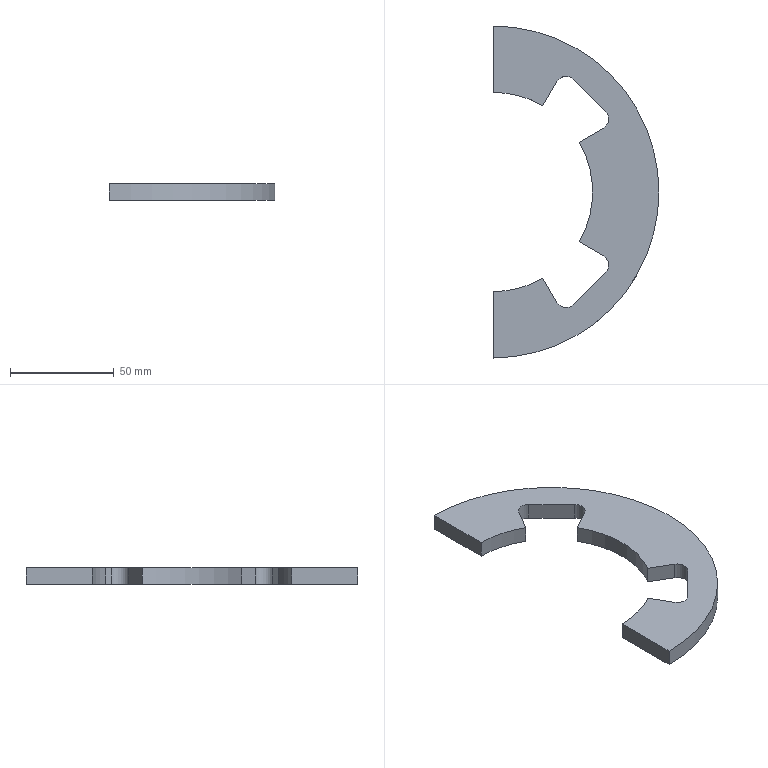Part | SolidWorks | features FlatPattern 1, SMBaseFlange 1, SheetMetal 1 | 1 solid | 18 faces | box 80 x 160 x 8 mm | volume 42936 mm3 | plane 10 | cylinder 8 | commonest cylinder face diameters 10 x4 96 x3 160 x1
STEP:
#1=CARTESIAN_POINT('',(125.,-80.,0.));
#2=VERTEX_POINT('',#1);
#3=CARTESIAN_POINT('',(125.,80.,0.));
#4=VERTEX_POINT('',#3);
#5=CARTESIAN_POINT('',(125.,0.,0.));
#6=DIRECTION('',(0.,0.,1.));
#7=DIRECTION('',(1.,0.,0.));
#8=AXIS2_PLACEMENT_3D('',#5,#6,#7);
#9=CIRCLE('',#8,80.);
#10=EDGE_CURVE('',#2,#4,#9,.T.);
#11=ORIENTED_EDGE('',*,*,#10,.T.);
#12=CARTESIAN_POINT('',(125.,80.,8.));
#13=VERTEX_POINT('',#12);
#14=CARTESIAN_POINT('',(125.,80.,8.));
#15=DIRECTION('',(0.,0.,-1.));
#16=VECTOR('',#15,1000.);
#17=LINE('',#14,#16);
#18=EDGE_CURVE('',#13,#4,#17,.T.);
#19=ORIENTED_EDGE('',*,*,#18,.F.);
#20=CARTESIAN_POINT('',(125.,-80.,8.));
#21=VERTEX_POINT('',#20);
#22=CARTESIAN_POINT('',(125.,0.,8.));
#23=DIRECTION('',(0.,0.,1.));
#24=DIRECTION('',(1.,0.,0.));
#25=AXIS2_PLACEMENT_3D('',#22,#23,#24);
#26=CIRCLE('',#25,80.);
#27=EDGE_CURVE('',#21,#13,#26,.T.);
#28=ORIENTED_EDGE('',*,*,#27,.F.);
#29=CARTESIAN_POINT('',(125.,-80.,8.));
#30=DIRECTION('',(0.,0.,-1.));
#31=VECTOR('',#30,1000.);
#32=LINE('',#29,#31);
#33=EDGE_CURVE('',#21,#2,#32,.T.);
#34=ORIENTED_EDGE('',*,*,#33,.T.);
#35=EDGE_LOOP('',(#11,#19,#28,#34));
#36=FACE_OUTER_BOUND('',#35,.T.);
#37=CARTESIAN_POINT('',(125.,0.,8.));
#38=DIRECTION('',(0.,0.,-1.));
#39=DIRECTION('',(-1.,0.,0.));
#40=AXIS2_PLACEMENT_3D('',#37,#38,#39);
#41=CYLINDRICAL_SURFACE('',#40,80.);
#42=ADVANCED_FACE('',(#36),#41,.T.);
#43=CARTESIAN_POINT('',(125.,48.,0.));
#44=VERTEX_POINT('',#43);
#45=CARTESIAN_POINT('',(125.,80.,0.));
#46=DIRECTION('',(0.,-1.,0.));
#47=VECTOR('',#46,1000.);
#48=LINE('',#45,#47);
#49=EDGE_CURVE('',#4,#44,#48,.T.);
#50=ORIENTED_EDGE('',*,*,#49,.T.);
#51=CARTESIAN_POINT('',(125.,48.,8.));
#52=VERTEX_POINT('',#51);
#53=CARTESIAN_POINT('',(125.,48.,8.));
#54=DIRECTION('',(0.,0.,-1.));
#55=VECTOR('',#54,1000.);
#56=LINE('',#53,#55);
#57=EDGE_CURVE('',#52,#44,#56,.T.);
#58=ORIENTED_EDGE('',*,*,#57,.F.);
#59=CARTESIAN_POINT('',(125.,80.,8.));
#60=DIRECTION('',(0.,-1.,0.));
#61=VECTOR('',#60,1000.);
#62=LINE('',#59,#61);
#63=EDGE_CURVE('',#13,#52,#62,.T.);
#64=ORIENTED_EDGE('',*,*,#63,.F.);
#65=ORIENTED_EDGE('',*,*,#18,.T.);
#66=EDGE_LOOP('',(#50,#58,#64,#65));
#67=FACE_OUTER_BOUND('',#66,.T.);
#68=CARTESIAN_POINT('',(125.,80.,8.));
#69=DIRECTION('',(1.,0.,0.));
#70=DIRECTION('',(0.,0.,-1.));
#71=AXIS2_PLACEMENT_3D('',#68,#69,#70);
#72=PLANE('',#71);
#73=ADVANCED_FACE('',(#67),#72,.F.);
#74=CARTESIAN_POINT('',(149.,41.569,0.));
#75=VERTEX_POINT('',#74);
#76=CARTESIAN_POINT('',(125.,0.,0.));
#77=DIRECTION('',(0.,0.,-1.));
#78=DIRECTION('',(1.,0.,0.));
#79=AXIS2_PLACEMENT_3D('',#76,#77,#78);
#80=CIRCLE('',#79,48.);
#81=EDGE_CURVE('',#44,#75,#80,.T.);
#82=ORIENTED_EDGE('',*,*,#81,.T.);
#83=CARTESIAN_POINT('',(149.,41.569,8.));
#84=VERTEX_POINT('',#83);
#85=CARTESIAN_POINT('',(149.,41.569,8.));
#86=DIRECTION('',(0.,0.,-1.));
#87=VECTOR('',#86,1000.);
#88=LINE('',#85,#87);
#89=EDGE_CURVE('',#84,#75,#88,.T.);
#90=ORIENTED_EDGE('',*,*,#89,.F.);
#91=CARTESIAN_POINT('',(125.,0.,8.));
#92=DIRECTION('',(0.,0.,-1.));
#93=DIRECTION('',(1.,0.,0.));
#94=AXIS2_PLACEMENT_3D('',#91,#92,#93);
#95=CIRCLE('',#94,48.);
#96=EDGE_CURVE('',#52,#84,#95,.T.);
#97=ORIENTED_EDGE('',*,*,#96,.F.);
#98=ORIENTED_EDGE('',*,*,#57,.T.);
#99=EDGE_LOOP('',(#82,#90,#97,#98));
#100=FACE_OUTER_BOUND('',#99,.T.);
#101=CARTESIAN_POINT('',(125.,0.,8.));
#102=DIRECTION('',(0.,0.,-1.));
#103=DIRECTION('',(-1.,0.,0.));
#104=AXIS2_PLACEMENT_3D('',#101,#102,#103);
#105=CYLINDRICAL_SURFACE('',#104,48.);
#106=ADVANCED_FACE('',(#100),#105,.F.);
#107=CARTESIAN_POINT('',(155.742,53.247,0.));
#108=VERTEX_POINT('',#107);
#109=CARTESIAN_POINT('',(155.742,53.247,0.));
#110=DIRECTION('',(0.5,0.866,0.));
#111=VECTOR('',#110,1000.);
#112=LINE('',#109,#111);
#113=EDGE_CURVE('',#75,#108,#112,.T.);
#114=ORIENTED_EDGE('',*,*,#113,.T.);
#115=CARTESIAN_POINT('',(155.742,53.247,8.));
#116=VERTEX_POINT('',#115);
#117=CARTESIAN_POINT('',(155.742,53.247,8.));
#118=DIRECTION('',(0.,0.,-1.));
#119=VECTOR('',#118,1000.);
#120=LINE('',#117,#119);
#121=EDGE_CURVE('',#116,#108,#120,.T.);
#122=ORIENTED_EDGE('',*,*,#121,.F.);
#123=CARTESIAN_POINT('',(155.742,53.247,8.));
#124=DIRECTION('',(0.5,0.866,0.));
#125=VECTOR('',#124,1000.);
#126=LINE('',#123,#125);
#127=EDGE_CURVE('',#84,#116,#126,.T.);
#128=ORIENTED_EDGE('',*,*,#127,.F.);
#129=ORIENTED_EDGE('',*,*,#89,.T.);
#130=EDGE_LOOP('',(#114,#122,#128,#129));
#131=FACE_OUTER_BOUND('',#130,.T.);
#132=CARTESIAN_POINT('',(155.742,53.247,8.));
#133=DIRECTION('',(-0.866,0.5,0.));
#134=DIRECTION('',(-0.5,-0.866,0.));
#135=AXIS2_PLACEMENT_3D('',#132,#133,#134);
#136=PLANE('',#135);
#137=ADVANCED_FACE('',(#131),#136,.F.);
#138=CARTESIAN_POINT('',(163.608,54.282,0.));
#139=VERTEX_POINT('',#138);
#140=CARTESIAN_POINT('',(160.072,50.747,0.));
#141=DIRECTION('',(0.,0.,-1.));
#142=DIRECTION('',(1.,0.,0.));
#143=AXIS2_PLACEMENT_3D('',#140,#141,#142);
#144=CIRCLE('',#143,5.);
#145=EDGE_CURVE('',#108,#139,#144,.T.);
#146=ORIENTED_EDGE('',*,*,#145,.T.);
#147=CARTESIAN_POINT('',(163.608,54.282,8.));
#148=VERTEX_POINT('',#147);
#149=CARTESIAN_POINT('',(163.608,54.282,8.));
#150=DIRECTION('',(0.,0.,-1.));
#151=VECTOR('',#150,1000.);
#152=LINE('',#149,#151);
#153=EDGE_CURVE('',#148,#139,#152,.T.);
#154=ORIENTED_EDGE('',*,*,#153,.F.);
#155=CARTESIAN_POINT('',(160.072,50.747,8.));
#156=DIRECTION('',(0.,0.,-1.));
#157=DIRECTION('',(1.,0.,0.));
#158=AXIS2_PLACEMENT_3D('',#155,#156,#157);
#159=CIRCLE('',#158,5.);
#160=EDGE_CURVE('',#116,#148,#159,.T.);
#161=ORIENTED_EDGE('',*,*,#160,.F.);
#162=ORIENTED_EDGE('',*,*,#121,.T.);
#163=EDGE_LOOP('',(#146,#154,#161,#162));
#164=FACE_OUTER_BOUND('',#163,.T.);
#165=CARTESIAN_POINT('',(160.072,50.747,8.));
#166=DIRECTION('',(0.,0.,-1.));
#167=DIRECTION('',(-1.,0.,0.));
#168=AXIS2_PLACEMENT_3D('',#165,#166,#167);
#169=CYLINDRICAL_SURFACE('',#168,5.);
#170=ADVANCED_FACE('',(#164),#169,.F.);
#171=CARTESIAN_POINT('',(179.282,38.608,0.));
#172=VERTEX_POINT('',#171);
#173=CARTESIAN_POINT('',(163.608,54.282,0.));
#174=DIRECTION('',(0.7071,-0.7071,0.));
#175=VECTOR('',#174,1000.);
#176=LINE('',#173,#175);
#177=EDGE_CURVE('',#139,#172,#176,.T.);
#178=ORIENTED_EDGE('',*,*,#177,.T.);
#179=CARTESIAN_POINT('',(179.282,38.608,8.));
#180=VERTEX_POINT('',#179);
#181=CARTESIAN_POINT('',(179.282,38.608,8.));
#182=DIRECTION('',(0.,0.,-1.));
#183=VECTOR('',#182,1000.);
#184=LINE('',#181,#183);
#185=EDGE_CURVE('',#180,#172,#184,.T.);
#186=ORIENTED_EDGE('',*,*,#185,.F.);
#187=CARTESIAN_POINT('',(163.608,54.282,8.));
#188=DIRECTION('',(0.7071,-0.7071,0.));
#189=VECTOR('',#188,1000.);
#190=LINE('',#187,#189);
#191=EDGE_CURVE('',#148,#180,#190,.T.);
#192=ORIENTED_EDGE('',*,*,#191,.F.);
#193=ORIENTED_EDGE('',*,*,#153,.T.);
#194=EDGE_LOOP('',(#178,#186,#192,#193));
#195=FACE_OUTER_BOUND('',#194,.T.);
#196=CARTESIAN_POINT('',(163.608,54.282,8.));
#197=DIRECTION('',(0.7071,0.7071,0.));
#198=DIRECTION('',(-0.7071,0.7071,0.));
#199=AXIS2_PLACEMENT_3D('',#196,#197,#198);
#200=PLANE('',#199);
#201=ADVANCED_FACE('',(#195),#200,.F.);
#202=CARTESIAN_POINT('',(178.247,30.742,0.));
#203=VERTEX_POINT('',#202);
#204=CARTESIAN_POINT('',(175.747,35.072,0.));
#205=DIRECTION('',(0.,0.,-1.));
#206=DIRECTION('',(1.,0.,0.));
#207=AXIS2_PLACEMENT_3D('',#204,#205,#206);
#208=CIRCLE('',#207,5.);
#209=EDGE_CURVE('',#172,#203,#208,.T.);
#210=ORIENTED_EDGE('',*,*,#209,.T.);
#211=CARTESIAN_POINT('',(178.247,30.742,8.));
#212=VERTEX_POINT('',#211);
#213=CARTESIAN_POINT('',(178.247,30.742,8.));
#214=DIRECTION('',(0.,0.,-1.));
#215=VECTOR('',#214,1000.);
#216=LINE('',#213,#215);
#217=EDGE_CURVE('',#212,#203,#216,.T.);
#218=ORIENTED_EDGE('',*,*,#217,.F.);
#219=CARTESIAN_POINT('',(175.747,35.072,8.));
#220=DIRECTION('',(0.,0.,-1.));
#221=DIRECTION('',(1.,0.,0.));
#222=AXIS2_PLACEMENT_3D('',#219,#220,#221);
#223=CIRCLE('',#222,5.);
#224=EDGE_CURVE('',#180,#212,#223,.T.);
#225=ORIENTED_EDGE('',*,*,#224,.F.);
#226=ORIENTED_EDGE('',*,*,#185,.T.);
#227=EDGE_LOOP('',(#210,#218,#225,#226));
#228=FACE_OUTER_BOUND('',#227,.T.);
#229=CARTESIAN_POINT('',(175.747,35.072,8.));
#230=DIRECTION('',(0.,0.,-1.));
#231=DIRECTION('',(-1.,0.,0.));
#232=AXIS2_PLACEMENT_3D('',#229,#230,#231);
#233=CYLINDRICAL_SURFACE('',#232,5.);
#234=ADVANCED_FACE('',(#228),#233,.F.);
#235=CARTESIAN_POINT('',(166.569,24.,0.));
#236=VERTEX_POINT('',#235);
#237=CARTESIAN_POINT('',(166.569,24.,0.));
#238=DIRECTION('',(-0.866,-0.5,0.));
#239=VECTOR('',#238,1000.);
#240=LINE('',#237,#239);
#241=EDGE_CURVE('',#203,#236,#240,.T.);
#242=ORIENTED_EDGE('',*,*,#241,.T.);
#243=CARTESIAN_POINT('',(166.569,24.,8.));
#244=VERTEX_POINT('',#243);
#245=CARTESIAN_POINT('',(166.569,24.,8.));
#246=DIRECTION('',(0.,0.,-1.));
#247=VECTOR('',#246,1000.);
#248=LINE('',#245,#247);
#249=EDGE_CURVE('',#244,#236,#248,.T.);
#250=ORIENTED_EDGE('',*,*,#249,.F.);
#251=CARTESIAN_POINT('',(166.569,24.,8.));
#252=DIRECTION('',(-0.866,-0.5,0.));
#253=VECTOR('',#252,1000.);
#254=LINE('',#251,#253);
#255=EDGE_CURVE('',#212,#244,#254,.T.);
#256=ORIENTED_EDGE('',*,*,#255,.F.);
#257=ORIENTED_EDGE('',*,*,#217,.T.);
#258=EDGE_LOOP('',(#242,#250,#256,#257));
#259=FACE_OUTER_BOUND('',#258,.T.);
#260=CARTESIAN_POINT('',(166.569,24.,8.));
#261=DIRECTION('',(0.5,-0.866,0.));
#262=DIRECTION('',(0.866,0.5,0.));
#263=AXIS2_PLACEMENT_3D('',#260,#261,#262);
#264=PLANE('',#263);
#265=ADVANCED_FACE('',(#259),#264,.F.);
#266=CARTESIAN_POINT('',(166.569,-24.,0.));
#267=VERTEX_POINT('',#266);
#268=CARTESIAN_POINT('',(125.,0.,0.));
#269=DIRECTION('',(0.,0.,-1.));
#270=DIRECTION('',(1.,0.,0.));
#271=AXIS2_PLACEMENT_3D('',#268,#269,#270);
#272=CIRCLE('',#271,48.);
#273=EDGE_CURVE('',#236,#267,#272,.T.);
#274=ORIENTED_EDGE('',*,*,#273,.T.);
#275=CARTESIAN_POINT('',(166.569,-24.,8.));
#276=VERTEX_POINT('',#275);
#277=CARTESIAN_POINT('',(166.569,-24.,8.));
#278=DIRECTION('',(0.,0.,-1.));
#279=VECTOR('',#278,1000.);
#280=LINE('',#277,#279);
#281=EDGE_CURVE('',#276,#267,#280,.T.);
#282=ORIENTED_EDGE('',*,*,#281,.F.);
#283=CARTESIAN_POINT('',(125.,0.,8.));
#284=DIRECTION('',(0.,0.,-1.));
#285=DIRECTION('',(1.,0.,0.));
#286=AXIS2_PLACEMENT_3D('',#283,#284,#285);
#287=CIRCLE('',#286,48.);
#288=EDGE_CURVE('',#244,#276,#287,.T.);
#289=ORIENTED_EDGE('',*,*,#288,.F.);
#290=ORIENTED_EDGE('',*,*,#249,.T.);
#291=EDGE_LOOP('',(#274,#282,#289,#290));
#292=FACE_OUTER_BOUND('',#291,.T.);
#293=CARTESIAN_POINT('',(125.,0.,8.));
#294=DIRECTION('',(0.,0.,-1.));
#295=DIRECTION('',(-1.,0.,0.));
#296=AXIS2_PLACEMENT_3D('',#293,#294,#295);
#297=CYLINDRICAL_SURFACE('',#296,48.);
#298=ADVANCED_FACE('',(#292),#297,.F.);
#299=CARTESIAN_POINT('',(178.247,-30.742,0.));
#300=VERTEX_POINT('',#299);
#301=CARTESIAN_POINT('',(166.569,-24.,0.));
#302=DIRECTION('',(0.866,-0.5,0.));
#303=VECTOR('',#302,1000.);
#304=LINE('',#301,#303);
#305=EDGE_CURVE('',#267,#300,#304,.T.);
#306=ORIENTED_EDGE('',*,*,#305,.T.);
#307=CARTESIAN_POINT('',(178.247,-30.742,8.));
#308=VERTEX_POINT('',#307);
#309=CARTESIAN_POINT('',(178.247,-30.742,8.));
#310=DIRECTION('',(0.,0.,-1.));
#311=VECTOR('',#310,1000.);
#312=LINE('',#309,#311);
#313=EDGE_CURVE('',#308,#300,#312,.T.);
#314=ORIENTED_EDGE('',*,*,#313,.F.);
#315=CARTESIAN_POINT('',(166.569,-24.,8.));
#316=DIRECTION('',(0.866,-0.5,0.));
#317=VECTOR('',#316,1000.);
#318=LINE('',#315,#317);
#319=EDGE_CURVE('',#276,#308,#318,.T.);
#320=ORIENTED_EDGE('',*,*,#319,.F.);
#321=ORIENTED_EDGE('',*,*,#281,.T.);
#322=EDGE_LOOP('',(#306,#314,#320,#321));
#323=FACE_OUTER_BOUND('',#322,.T.);
#324=CARTESIAN_POINT('',(166.569,-24.,8.));
#325=DIRECTION('',(0.5,0.866,0.));
#326=DIRECTION('',(-0.866,0.5,0.));
#327=AXIS2_PLACEMENT_3D('',#324,#325,#326);
#328=PLANE('',#327);
#329=ADVANCED_FACE('',(#323),#328,.F.);
#330=CARTESIAN_POINT('',(179.282,-38.608,0.));
#331=VERTEX_POINT('',#330);
#332=CARTESIAN_POINT('',(175.747,-35.072,0.));
#333=DIRECTION('',(0.,0.,-1.));
#334=DIRECTION('',(-1.,0.,0.));
#335=AXIS2_PLACEMENT_3D('',#332,#333,#334);
#336=CIRCLE('',#335,5.);
#337=EDGE_CURVE('',#300,#331,#336,.T.);
#338=ORIENTED_EDGE('',*,*,#337,.T.);
#339=CARTESIAN_POINT('',(179.282,-38.608,8.));
#340=VERTEX_POINT('',#339);
#341=CARTESIAN_POINT('',(179.282,-38.608,8.));
#342=DIRECTION('',(0.,0.,-1.));
#343=VECTOR('',#342,1000.);
#344=LINE('',#341,#343);
#345=EDGE_CURVE('',#340,#331,#344,.T.);
#346=ORIENTED_EDGE('',*,*,#345,.F.);
#347=CARTESIAN_POINT('',(175.747,-35.072,8.));
#348=DIRECTION('',(0.,0.,-1.));
#349=DIRECTION('',(-1.,0.,0.));
#350=AXIS2_PLACEMENT_3D('',#347,#348,#349);
#351=CIRCLE('',#350,5.);
#352=EDGE_CURVE('',#308,#340,#351,.T.);
#353=ORIENTED_EDGE('',*,*,#352,.F.);
#354=ORIENTED_EDGE('',*,*,#313,.T.);
#355=EDGE_LOOP('',(#338,#346,#353,#354));
#356=FACE_OUTER_BOUND('',#355,.T.);
#357=CARTESIAN_POINT('',(175.747,-35.072,8.));
#358=DIRECTION('',(0.,0.,-1.));
#359=DIRECTION('',(-1.,0.,0.));
#360=AXIS2_PLACEMENT_3D('',#357,#358,#359);
#361=CYLINDRICAL_SURFACE('',#360,5.);
#362=ADVANCED_FACE('',(#356),#361,.F.);
#363=CARTESIAN_POINT('',(163.608,-54.282,0.));
#364=VERTEX_POINT('',#363);
#365=CARTESIAN_POINT('',(163.608,-54.282,0.));
#366=DIRECTION('',(-0.7071,-0.7071,0.));
#367=VECTOR('',#366,1000.);
#368=LINE('',#365,#367);
#369=EDGE_CURVE('',#331,#364,#368,.T.);
#370=ORIENTED_EDGE('',*,*,#369,.T.);
#371=CARTESIAN_POINT('',(163.608,-54.282,8.));
#372=VERTEX_POINT('',#371);
#373=CARTESIAN_POINT('',(163.608,-54.282,8.));
#374=DIRECTION('',(0.,0.,-1.));
#375=VECTOR('',#374,1000.);
#376=LINE('',#373,#375);
#377=EDGE_CURVE('',#372,#364,#376,.T.);
#378=ORIENTED_EDGE('',*,*,#377,.F.);
#379=CARTESIAN_POINT('',(163.608,-54.282,8.));
#380=DIRECTION('',(-0.7071,-0.7071,0.));
#381=VECTOR('',#380,1000.);
#382=LINE('',#379,#381);
#383=EDGE_CURVE('',#340,#372,#382,.T.);
#384=ORIENTED_EDGE('',*,*,#383,.F.);
#385=ORIENTED_EDGE('',*,*,#345,.T.);
#386=EDGE_LOOP('',(#370,#378,#384,#385));
#387=FACE_OUTER_BOUND('',#386,.T.);
#388=CARTESIAN_POINT('',(163.608,-54.282,8.));
#389=DIRECTION('',(0.7071,-0.7071,0.));
#390=DIRECTION('',(0.7071,0.7071,0.));
#391=AXIS2_PLACEMENT_3D('',#388,#389,#390);
#392=PLANE('',#391);
#393=ADVANCED_FACE('',(#387),#392,.F.);
#394=CARTESIAN_POINT('',(155.742,-53.247,0.));
#395=VERTEX_POINT('',#394);
#396=CARTESIAN_POINT('',(160.072,-50.747,0.));
#397=DIRECTION('',(0.,0.,-1.));
#398=DIRECTION('',(-1.,0.,0.));
#399=AXIS2_PLACEMENT_3D('',#396,#397,#398);
#400=CIRCLE('',#399,5.);
#401=EDGE_CURVE('',#364,#395,#400,.T.);
#402=ORIENTED_EDGE('',*,*,#401,.T.);
#403=CARTESIAN_POINT('',(155.742,-53.247,8.));
#404=VERTEX_POINT('',#403);
#405=CARTESIAN_POINT('',(155.742,-53.247,8.));
#406=DIRECTION('',(0.,0.,-1.));
#407=VECTOR('',#406,1000.);
#408=LINE('',#405,#407);
#409=EDGE_CURVE('',#404,#395,#408,.T.);
#410=ORIENTED_EDGE('',*,*,#409,.F.);
#411=CARTESIAN_POINT('',(160.072,-50.747,8.));
#412=DIRECTION('',(0.,0.,-1.));
#413=DIRECTION('',(-1.,0.,0.));
#414=AXIS2_PLACEMENT_3D('',#411,#412,#413);
#415=CIRCLE('',#414,5.);
#416=EDGE_CURVE('',#372,#404,#415,.T.);
#417=ORIENTED_EDGE('',*,*,#416,.F.);
#418=ORIENTED_EDGE('',*,*,#377,.T.);
#419=EDGE_LOOP('',(#402,#410,#417,#418));
#420=FACE_OUTER_BOUND('',#419,.T.);
#421=CARTESIAN_POINT('',(160.072,-50.747,8.));
#422=DIRECTION('',(0.,0.,-1.));
#423=DIRECTION('',(-1.,0.,0.));
#424=AXIS2_PLACEMENT_3D('',#421,#422,#423);
#425=CYLINDRICAL_SURFACE('',#424,5.);
#426=ADVANCED_FACE('',(#420),#425,.F.);
#427=CARTESIAN_POINT('',(149.,-41.569,0.));
#428=VERTEX_POINT('',#427);
#429=CARTESIAN_POINT('',(155.742,-53.247,0.));
#430=DIRECTION('',(-0.5,0.866,0.));
#431=VECTOR('',#430,1000.);
#432=LINE('',#429,#431);
#433=EDGE_CURVE('',#395,#428,#432,.T.);
#434=ORIENTED_EDGE('',*,*,#433,.T.);
#435=CARTESIAN_POINT('',(149.,-41.569,8.));
#436=VERTEX_POINT('',#435);
#437=CARTESIAN_POINT('',(149.,-41.569,8.));
#438=DIRECTION('',(0.,0.,-1.));
#439=VECTOR('',#438,1000.);
#440=LINE('',#437,#439);
#441=EDGE_CURVE('',#436,#428,#440,.T.);
#442=ORIENTED_EDGE('',*,*,#441,.F.);
#443=CARTESIAN_POINT('',(155.742,-53.247,8.));
#444=DIRECTION('',(-0.5,0.866,0.));
#445=VECTOR('',#444,1000.);
#446=LINE('',#443,#445);
#447=EDGE_CURVE('',#404,#436,#446,.T.);
#448=ORIENTED_EDGE('',*,*,#447,.F.);
#449=ORIENTED_EDGE('',*,*,#409,.T.);
#450=EDGE_LOOP('',(#434,#442,#448,#449));
#451=FACE_OUTER_BOUND('',#450,.T.);
#452=CARTESIAN_POINT('',(155.742,-53.247,8.));
#453=DIRECTION('',(-0.866,-0.5,0.));
#454=DIRECTION('',(0.5,-0.866,0.));
#455=AXIS2_PLACEMENT_3D('',#452,#453,#454);
#456=PLANE('',#455);
#457=ADVANCED_FACE('',(#451),#456,.F.);
#458=CARTESIAN_POINT('',(125.,-48.,0.));
#459=VERTEX_POINT('',#458);
#460=CARTESIAN_POINT('',(125.,0.,0.));
#461=DIRECTION('',(0.,0.,-1.));
#462=DIRECTION('',(1.,0.,0.));
#463=AXIS2_PLACEMENT_3D('',#460,#461,#462);
#464=CIRCLE('',#463,48.);
#465=EDGE_CURVE('',#428,#459,#464,.T.);
#466=ORIENTED_EDGE('',*,*,#465,.T.);
#467=CARTESIAN_POINT('',(125.,-48.,8.));
#468=VERTEX_POINT('',#467);
#469=CARTESIAN_POINT('',(125.,-48.,8.));
#470=DIRECTION('',(0.,0.,-1.));
#471=VECTOR('',#470,1000.);
#472=LINE('',#469,#471);
#473=EDGE_CURVE('',#468,#459,#472,.T.);
#474=ORIENTED_EDGE('',*,*,#473,.F.);
#475=CARTESIAN_POINT('',(125.,0.,8.));
#476=DIRECTION('',(0.,0.,-1.));
#477=DIRECTION('',(1.,0.,0.));
#478=AXIS2_PLACEMENT_3D('',#475,#476,#477);
#479=CIRCLE('',#478,48.);
#480=EDGE_CURVE('',#436,#468,#479,.T.);
#481=ORIENTED_EDGE('',*,*,#480,.F.);
#482=ORIENTED_EDGE('',*,*,#441,.T.);
#483=EDGE_LOOP('',(#466,#474,#481,#482));
#484=FACE_OUTER_BOUND('',#483,.T.);
#485=CARTESIAN_POINT('',(125.,0.,8.));
#486=DIRECTION('',(0.,0.,-1.));
#487=DIRECTION('',(-1.,0.,0.));
#488=AXIS2_PLACEMENT_3D('',#485,#486,#487);
#489=CYLINDRICAL_SURFACE('',#488,48.);
#490=ADVANCED_FACE('',(#484),#489,.F.);
#491=CARTESIAN_POINT('',(125.,-48.,0.));
#492=DIRECTION('',(0.,-1.,0.));
#493=VECTOR('',#492,1000.);
#494=LINE('',#491,#493);
#495=EDGE_CURVE('',#459,#2,#494,.T.);
#496=ORIENTED_EDGE('',*,*,#495,.T.);
#497=ORIENTED_EDGE('',*,*,#33,.F.);
#498=CARTESIAN_POINT('',(125.,-48.,8.));
#499=DIRECTION('',(0.,-1.,0.));
#500=VECTOR('',#499,1000.);
#501=LINE('',#498,#500);
#502=EDGE_CURVE('',#468,#21,#501,.T.);
#503=ORIENTED_EDGE('',*,*,#502,.F.);
#504=ORIENTED_EDGE('',*,*,#473,.T.);
#505=EDGE_LOOP('',(#496,#497,#503,#504));
#506=FACE_OUTER_BOUND('',#505,.T.);
#507=CARTESIAN_POINT('',(125.,-48.,8.));
#508=DIRECTION('',(1.,0.,0.));
#509=DIRECTION('',(0.,0.,-1.));
#510=AXIS2_PLACEMENT_3D('',#507,#508,#509);
#511=PLANE('',#510);
#512=ADVANCED_FACE('',(#506),#511,.F.);
#513=ORIENTED_EDGE('',*,*,#27,.T.);
#514=ORIENTED_EDGE('',*,*,#63,.T.);
#515=ORIENTED_EDGE('',*,*,#96,.T.);
#516=ORIENTED_EDGE('',*,*,#127,.T.);
#517=ORIENTED_EDGE('',*,*,#160,.T.);
#518=ORIENTED_EDGE('',*,*,#191,.T.);
#519=ORIENTED_EDGE('',*,*,#224,.T.);
#520=ORIENTED_EDGE('',*,*,#255,.T.);
#521=ORIENTED_EDGE('',*,*,#288,.T.);
#522=ORIENTED_EDGE('',*,*,#319,.T.);
#523=ORIENTED_EDGE('',*,*,#352,.T.);
#524=ORIENTED_EDGE('',*,*,#383,.T.);
#525=ORIENTED_EDGE('',*,*,#416,.T.);
#526=ORIENTED_EDGE('',*,*,#447,.T.);
#527=ORIENTED_EDGE('',*,*,#480,.T.);
#528=ORIENTED_EDGE('',*,*,#502,.T.);
#529=EDGE_LOOP('',(#513,#514,#515,#516,#517,#518,#519,#520,#521,#522,#523,#524,#525,#526,#527,#528));
#530=FACE_OUTER_BOUND('',#529,.T.);
#531=CARTESIAN_POINT('',(125.,0.,8.));
#532=DIRECTION('',(0.,0.,1.));
#533=DIRECTION('',(1.,0.,0.));
#534=AXIS2_PLACEMENT_3D('',#531,#532,#533);
#535=PLANE('',#534);
#536=ADVANCED_FACE('',(#530),#535,.T.);
#537=ORIENTED_EDGE('',*,*,#10,.F.);
#538=ORIENTED_EDGE('',*,*,#495,.F.);
#539=ORIENTED_EDGE('',*,*,#465,.F.);
#540=ORIENTED_EDGE('',*,*,#433,.F.);
#541=ORIENTED_EDGE('',*,*,#401,.F.);
#542=ORIENTED_EDGE('',*,*,#369,.F.);
#543=ORIENTED_EDGE('',*,*,#337,.F.);
#544=ORIENTED_EDGE('',*,*,#305,.F.);
#545=ORIENTED_EDGE('',*,*,#273,.F.);
#546=ORIENTED_EDGE('',*,*,#241,.F.);
#547=ORIENTED_EDGE('',*,*,#209,.F.);
#548=ORIENTED_EDGE('',*,*,#177,.F.);
#549=ORIENTED_EDGE('',*,*,#145,.F.);
#550=ORIENTED_EDGE('',*,*,#113,.F.);
#551=ORIENTED_EDGE('',*,*,#81,.F.);
#552=ORIENTED_EDGE('',*,*,#49,.F.);
#553=EDGE_LOOP('',(#537,#538,#539,#540,#541,#542,#543,#544,#545,#546,#547,#548,#549,#550,#551,#552));
#554=FACE_OUTER_BOUND('',#553,.T.);
#555=CARTESIAN_POINT('',(125.,0.,0.));
#556=DIRECTION('',(0.,0.,1.));
#557=DIRECTION('',(1.,0.,0.));
#558=AXIS2_PLACEMENT_3D('',#555,#556,#557);
#559=PLANE('',#558);
#560=ADVANCED_FACE('',(#554),#559,.F.);
#561=CLOSED_SHELL('',(#42,#73,#106,#137,#170,#201,#234,#265,#298,#329,#362,#393,#426,#457,#490,#512,#536,#560));
#562=MANIFOLD_SOLID_BREP('',#561);
#563=CARTESIAN_POINT('',(0.,0.,0.));
#564=DIRECTION('',(0.,0.,1.));
#565=DIRECTION('',(1.,0.,0.));
#566=AXIS2_PLACEMENT_3D('',#563,#564,#565);
#567=(LENGTH_UNIT()NAMED_UNIT(*)SI_UNIT(.MILLI.,.METRE.));
#568=UNCERTAINTY_MEASURE_WITH_UNIT(LENGTH_MEASURE(0.00001),#567,'','');
#569=(NAMED_UNIT(*)PLANE_ANGLE_UNIT()SI_UNIT($,.RADIAN.));
#570=(NAMED_UNIT(*)SI_UNIT($,.STERADIAN.)SOLID_ANGLE_UNIT());
#571=(GEOMETRIC_REPRESENTATION_CONTEXT(3)GLOBAL_UNCERTAINTY_ASSIGNED_CONTEXT((#568))GLOBAL_UNIT_ASSIGNED_CONTEXT((#567,#569,#570))REPRESENTATION_CONTEXT('',''));
#572=ADVANCED_BREP_SHAPE_REPRESENTATION('',(#562,#566),#571);